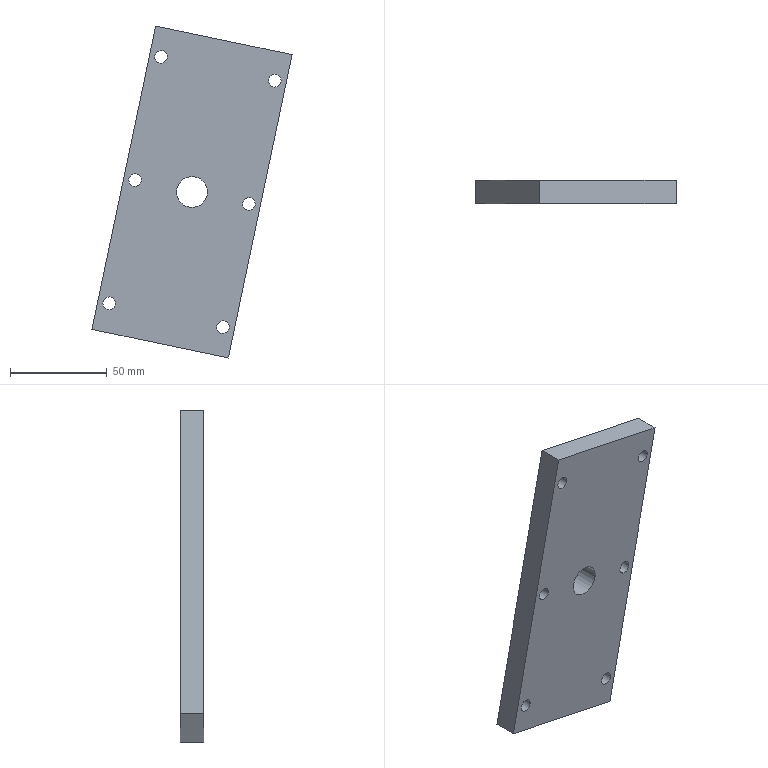Part | STEP file | SN10_007_001-03_PLACA | 1 solid | 13 faces | box 103.364 x 12 x 171.387 mm | volume 133438 mm3 | cylinder 7 | plane 6 | commonest cylinder face diameters 6.5 x6 16 x1
STEP:
#1=CARTESIAN_POINT('',(0.,0.,0.));
#2=DIRECTION('',(0.,0.,1.));
#3=DIRECTION('',(1.,0.,0.));
#4=AXIS2_PLACEMENT_3D('',#1,#2,#3);
#5=CARTESIAN_POINT('',(-608.399,-875.15,536.206));
#6=VERTEX_POINT('',#5);
#7=CARTESIAN_POINT('',(-592.741,-875.15,532.916));
#8=VERTEX_POINT('',#7);
#9=CARTESIAN_POINT('',(-600.57,-875.15,534.561));
#10=DIRECTION('',(0.,1.,0.));
#11=DIRECTION('',(0.9786,0.,-0.2056));
#12=AXIS2_PLACEMENT_3D('',#9,#10,#11);
#13=CIRCLE('',#12,8.);
#14=CARTESIAN_POINT('',(-600.57,-1063.653,534.561));
#15=DIRECTION('',(0.,1.,0.));
#16=DIRECTION('',(0.9786,0.,-0.2056));
#17=AXIS2_PLACEMENT_3D('',#14,#15,#16);
#18=CYLINDRICAL_SURFACE('',#17,8.);
#19=CARTESIAN_POINT('',(0.,188.503));
#20=DIRECTION('',(1.,0.));
#21=VECTOR('',#20,1.);
#22=LINE('',#19,#21);
#23=(GEOMETRIC_REPRESENTATION_CONTEXT(2)PARAMETRIC_REPRESENTATION_CONTEXT()REPRESENTATION_CONTEXT('',''));
#24=DEFINITIONAL_REPRESENTATION('',(#22),#23);
#25=PCURVE('',#18,#24);
#26=CARTESIAN_POINT('',(0.,-875.15,0.));
#27=DIRECTION('',(0.,1.,0.));
#28=DIRECTION('',(0.,0.,1.));
#29=AXIS2_PLACEMENT_3D('',#26,#27,#28);
#30=PLANE('',#29);
#31=CARTESIAN_POINT('',(534.561,-600.57));
#32=DIRECTION('',(-0.2056,0.9786));
#33=AXIS2_PLACEMENT_2D('',#31,#32);
#34=CIRCLE('',#33,8.);
#35=(GEOMETRIC_REPRESENTATION_CONTEXT(2)PARAMETRIC_REPRESENTATION_CONTEXT()REPRESENTATION_CONTEXT('',''));
#36=DEFINITIONAL_REPRESENTATION('',(#34),#35);
#37=PCURVE('',#30,#36);
#38=SURFACE_CURVE('',#13,(#25,#37),.PCURVE_S1.);
#39=EDGE_CURVE('',#6,#8,#38,.T.);
#40=ORIENTED_EDGE('',*,*,#39,.T.);
#41=CARTESIAN_POINT('',(-592.741,-863.15,532.916));
#42=VERTEX_POINT('',#41);
#43=CARTESIAN_POINT('',(-592.741,-875.15,532.916));
#44=CARTESIAN_POINT('',(-592.741,-863.15,532.916));
#45=B_SPLINE_CURVE_WITH_KNOTS('',1,(#43,#44),.UNSPECIFIED.,.F.,.F.,(2,2),(188.503,200.503),.PIECEWISE_BEZIER_KNOTS.);
#46=CARTESIAN_POINT('',(6.283,0.));
#47=DIRECTION('',(0.,1.));
#48=VECTOR('',#47,1.);
#49=LINE('',#46,#48);
#50=(GEOMETRIC_REPRESENTATION_CONTEXT(2)PARAMETRIC_REPRESENTATION_CONTEXT()REPRESENTATION_CONTEXT('',''));
#51=DEFINITIONAL_REPRESENTATION('',(#49),#50);
#52=PCURVE('',#18,#51);
#53=CARTESIAN_POINT('',(0.,0.));
#54=DIRECTION('',(0.,1.));
#55=VECTOR('',#54,1.);
#56=LINE('',#53,#55);
#57=(GEOMETRIC_REPRESENTATION_CONTEXT(2)PARAMETRIC_REPRESENTATION_CONTEXT()REPRESENTATION_CONTEXT('',''));
#58=DEFINITIONAL_REPRESENTATION('',(#56),#57);
#59=PCURVE('',#18,#58);
#60=SEAM_CURVE('',#45,(#52,#59),.PCURVE_S1.);
#61=EDGE_CURVE('',#8,#42,#60,.T.);
#62=ORIENTED_EDGE('',*,*,#61,.T.);
#63=CARTESIAN_POINT('',(-600.57,-863.15,534.561));
#64=DIRECTION('',(0.,-1.,0.));
#65=DIRECTION('',(0.9786,0.,-0.2056));
#66=AXIS2_PLACEMENT_3D('',#63,#64,#65);
#67=CIRCLE('',#66,8.);
#68=CARTESIAN_POINT('',(6.283,200.503));
#69=DIRECTION('',(-1.,0.));
#70=VECTOR('',#69,1.);
#71=LINE('',#68,#70);
#72=(GEOMETRIC_REPRESENTATION_CONTEXT(2)PARAMETRIC_REPRESENTATION_CONTEXT()REPRESENTATION_CONTEXT('',''));
#73=DEFINITIONAL_REPRESENTATION('',(#71),#72);
#74=PCURVE('',#18,#73);
#75=CARTESIAN_POINT('',(-541.059,-863.15,603.803));
#76=DIRECTION('',(0.,1.,0.));
#77=DIRECTION('',(0.,0.,1.));
#78=AXIS2_PLACEMENT_3D('',#75,#76,#77);
#79=PLANE('',#78);
#80=CARTESIAN_POINT('',(-70.887,-51.682));
#81=CARTESIAN_POINT('',(-57.327,-48.833));
#82=CARTESIAN_POINT('',(-61.639,-62.001));
#83=CARTESIAN_POINT('',(-65.952,-75.169));
#84=CARTESIAN_POINT('',(-75.199,-64.85));
#85=CARTESIAN_POINT('',(-84.447,-54.532));
#86=CARTESIAN_POINT('',(-70.887,-51.682));
#87=(BOUNDED_CURVE()B_SPLINE_CURVE(2,(#80,#81,#82,#83,#84,#85,#86),.UNSPECIFIED.,.T.,.F.)B_SPLINE_CURVE_WITH_KNOTS((1,2,2,2,2,1),(-2.094,0.,2.094,4.189,6.283,8.378),.UNSPECIFIED.)CURVE()GEOMETRIC_REPRESENTATION_ITEM()RATIONAL_B_SPLINE_CURVE((1.,0.5,1.,0.5,1.,0.5,1.))REPRESENTATION_ITEM(''));
#88=(GEOMETRIC_REPRESENTATION_CONTEXT(2)PARAMETRIC_REPRESENTATION_CONTEXT()REPRESENTATION_CONTEXT('',''));
#89=DEFINITIONAL_REPRESENTATION('',(#87),#88);
#90=PCURVE('',#79,#89);
#91=SURFACE_CURVE('',#67,(#74,#90),.PCURVE_S1.);
#92=EDGE_CURVE('',#42,#42,#91,.T.);
#93=ORIENTED_EDGE('',*,*,#92,.T.);
#94=ORIENTED_EDGE('',*,*,#61,.F.);
#95=CARTESIAN_POINT('',(-600.57,-875.15,534.561));
#96=DIRECTION('',(0.,1.,0.));
#97=DIRECTION('',(0.9786,0.,-0.2056));
#98=AXIS2_PLACEMENT_3D('',#95,#96,#97);
#99=CIRCLE('',#98,8.);
#100=CARTESIAN_POINT('',(-6.283,188.503));
#101=DIRECTION('',(1.,0.));
#102=VECTOR('',#101,1.);
#103=LINE('',#100,#102);
#104=(GEOMETRIC_REPRESENTATION_CONTEXT(2)PARAMETRIC_REPRESENTATION_CONTEXT()REPRESENTATION_CONTEXT('',''));
#105=DEFINITIONAL_REPRESENTATION('',(#103),#104);
#106=PCURVE('',#18,#105);
#107=CARTESIAN_POINT('',(534.561,-600.57));
#108=DIRECTION('',(-0.2056,0.9786));
#109=AXIS2_PLACEMENT_2D('',#107,#108);
#110=CIRCLE('',#109,8.);
#111=(GEOMETRIC_REPRESENTATION_CONTEXT(2)PARAMETRIC_REPRESENTATION_CONTEXT()REPRESENTATION_CONTEXT('',''));
#112=DEFINITIONAL_REPRESENTATION('',(#110),#111);
#113=PCURVE('',#30,#112);
#114=SURFACE_CURVE('',#99,(#106,#113),.PCURVE_S1.);
#115=EDGE_CURVE('',#8,#6,#114,.T.);
#116=ORIENTED_EDGE('',*,*,#115,.T.);
#117=EDGE_LOOP('',(#40,#62,#93,#94,#116));
#118=FACE_BOUND('',#117,.F.);
#119=ADVANCED_FACE('',(#118),#18,.F.);
#120=CARTESIAN_POINT('',(-587.759,-863.15,465.449));
#121=VERTEX_POINT('',#120);
#122=CARTESIAN_POINT('',(-581.398,-863.15,464.113));
#123=VERTEX_POINT('',#122);
#124=CARTESIAN_POINT('',(-584.578,-863.15,464.781));
#125=DIRECTION('',(0.,-1.,0.));
#126=DIRECTION('',(0.9786,0.,-0.2056));
#127=AXIS2_PLACEMENT_3D('',#124,#125,#126);
#128=CIRCLE('',#127,3.25);
#129=CARTESIAN_POINT('',(-584.578,-674.647,464.781));
#130=DIRECTION('',(0.,-1.,0.));
#131=DIRECTION('',(0.9786,0.,-0.2056));
#132=AXIS2_PLACEMENT_3D('',#129,#130,#131);
#133=CYLINDRICAL_SURFACE('',#132,3.25);
#134=CARTESIAN_POINT('',(0.,188.503));
#135=DIRECTION('',(1.,0.));
#136=VECTOR('',#135,1.);
#137=LINE('',#134,#136);
#138=(GEOMETRIC_REPRESENTATION_CONTEXT(2)PARAMETRIC_REPRESENTATION_CONTEXT()REPRESENTATION_CONTEXT('',''));
#139=DEFINITIONAL_REPRESENTATION('',(#137),#138);
#140=PCURVE('',#133,#139);
#141=CARTESIAN_POINT('',(-139.69,-40.339));
#142=CARTESIAN_POINT('',(-134.181,-39.181));
#143=CARTESIAN_POINT('',(-135.933,-44.531));
#144=CARTESIAN_POINT('',(-137.685,-49.88));
#145=CARTESIAN_POINT('',(-141.442,-45.688));
#146=CARTESIAN_POINT('',(-145.199,-41.496));
#147=CARTESIAN_POINT('',(-139.69,-40.339));
#148=(BOUNDED_CURVE()B_SPLINE_CURVE(2,(#141,#142,#143,#144,#145,#146,#147),.UNSPECIFIED.,.T.,.F.)B_SPLINE_CURVE_WITH_KNOTS((1,2,2,2,2,1),(-2.094,0.,2.094,4.189,6.283,8.378),.UNSPECIFIED.)CURVE()GEOMETRIC_REPRESENTATION_ITEM()RATIONAL_B_SPLINE_CURVE((1.,0.5,1.,0.5,1.,0.5,1.))REPRESENTATION_ITEM(''));
#149=(GEOMETRIC_REPRESENTATION_CONTEXT(2)PARAMETRIC_REPRESENTATION_CONTEXT()REPRESENTATION_CONTEXT('',''));
#150=DEFINITIONAL_REPRESENTATION('',(#148),#149);
#151=PCURVE('',#79,#150);
#152=SURFACE_CURVE('',#128,(#140,#151),.PCURVE_S1.);
#153=EDGE_CURVE('',#121,#123,#152,.T.);
#154=ORIENTED_EDGE('',*,*,#153,.T.);
#155=CARTESIAN_POINT('',(-581.398,-875.15,464.113));
#156=VERTEX_POINT('',#155);
#157=CARTESIAN_POINT('',(-581.398,-863.15,464.113));
#158=CARTESIAN_POINT('',(-581.398,-875.15,464.113));
#159=B_SPLINE_CURVE_WITH_KNOTS('',1,(#157,#158),.UNSPECIFIED.,.F.,.F.,(2,2),(188.503,200.503),.PIECEWISE_BEZIER_KNOTS.);
#160=CARTESIAN_POINT('',(6.283,0.));
#161=DIRECTION('',(0.,1.));
#162=VECTOR('',#161,1.);
#163=LINE('',#160,#162);
#164=(GEOMETRIC_REPRESENTATION_CONTEXT(2)PARAMETRIC_REPRESENTATION_CONTEXT()REPRESENTATION_CONTEXT('',''));
#165=DEFINITIONAL_REPRESENTATION('',(#163),#164);
#166=PCURVE('',#133,#165);
#167=CARTESIAN_POINT('',(0.,0.));
#168=DIRECTION('',(0.,1.));
#169=VECTOR('',#168,1.);
#170=LINE('',#167,#169);
#171=(GEOMETRIC_REPRESENTATION_CONTEXT(2)PARAMETRIC_REPRESENTATION_CONTEXT()REPRESENTATION_CONTEXT('',''));
#172=DEFINITIONAL_REPRESENTATION('',(#170),#171);
#173=PCURVE('',#133,#172);
#174=SEAM_CURVE('',#159,(#166,#173),.PCURVE_S1.);
#175=EDGE_CURVE('',#123,#156,#174,.T.);
#176=ORIENTED_EDGE('',*,*,#175,.T.);
#177=CARTESIAN_POINT('',(-584.578,-875.15,464.781));
#178=DIRECTION('',(0.,1.,0.));
#179=DIRECTION('',(0.9786,0.,-0.2056));
#180=AXIS2_PLACEMENT_3D('',#177,#178,#179);
#181=CIRCLE('',#180,3.25);
#182=CARTESIAN_POINT('',(6.283,200.503));
#183=DIRECTION('',(-1.,0.));
#184=VECTOR('',#183,1.);
#185=LINE('',#182,#184);
#186=(GEOMETRIC_REPRESENTATION_CONTEXT(2)PARAMETRIC_REPRESENTATION_CONTEXT()REPRESENTATION_CONTEXT('',''));
#187=DEFINITIONAL_REPRESENTATION('',(#185),#186);
#188=PCURVE('',#133,#187);
#189=CARTESIAN_POINT('',(464.781,-584.578));
#190=DIRECTION('',(-0.2056,0.9786));
#191=AXIS2_PLACEMENT_2D('',#189,#190);
#192=CIRCLE('',#191,3.25);
#193=(GEOMETRIC_REPRESENTATION_CONTEXT(2)PARAMETRIC_REPRESENTATION_CONTEXT()REPRESENTATION_CONTEXT('',''));
#194=DEFINITIONAL_REPRESENTATION('',(#192),#193);
#195=PCURVE('',#30,#194);
#196=SURFACE_CURVE('',#181,(#188,#195),.PCURVE_S1.);
#197=EDGE_CURVE('',#156,#156,#196,.T.);
#198=ORIENTED_EDGE('',*,*,#197,.T.);
#199=ORIENTED_EDGE('',*,*,#175,.F.);
#200=CARTESIAN_POINT('',(-584.578,-863.15,464.781));
#201=DIRECTION('',(0.,-1.,0.));
#202=DIRECTION('',(0.9786,0.,-0.2056));
#203=AXIS2_PLACEMENT_3D('',#200,#201,#202);
#204=CIRCLE('',#203,3.25);
#205=CARTESIAN_POINT('',(-6.283,188.503));
#206=DIRECTION('',(1.,0.));
#207=VECTOR('',#206,1.);
#208=LINE('',#205,#207);
#209=(GEOMETRIC_REPRESENTATION_CONTEXT(2)PARAMETRIC_REPRESENTATION_CONTEXT()REPRESENTATION_CONTEXT('',''));
#210=DEFINITIONAL_REPRESENTATION('',(#208),#209);
#211=PCURVE('',#133,#210);
#212=CARTESIAN_POINT('',(-139.69,-40.339));
#213=CARTESIAN_POINT('',(-134.181,-39.181));
#214=CARTESIAN_POINT('',(-135.933,-44.531));
#215=CARTESIAN_POINT('',(-137.685,-49.88));
#216=CARTESIAN_POINT('',(-141.442,-45.688));
#217=CARTESIAN_POINT('',(-145.199,-41.496));
#218=CARTESIAN_POINT('',(-139.69,-40.339));
#219=(BOUNDED_CURVE()B_SPLINE_CURVE(2,(#212,#213,#214,#215,#216,#217,#218),.UNSPECIFIED.,.T.,.F.)B_SPLINE_CURVE_WITH_KNOTS((1,2,2,2,2,1),(-2.094,0.,2.094,4.189,6.283,8.378),.UNSPECIFIED.)CURVE()GEOMETRIC_REPRESENTATION_ITEM()RATIONAL_B_SPLINE_CURVE((1.,0.5,1.,0.5,1.,0.5,1.))REPRESENTATION_ITEM(''));
#220=(GEOMETRIC_REPRESENTATION_CONTEXT(2)PARAMETRIC_REPRESENTATION_CONTEXT()REPRESENTATION_CONTEXT('',''));
#221=DEFINITIONAL_REPRESENTATION('',(#219),#220);
#222=PCURVE('',#79,#221);
#223=SURFACE_CURVE('',#204,(#211,#222),.PCURVE_S1.);
#224=EDGE_CURVE('',#123,#121,#223,.T.);
#225=ORIENTED_EDGE('',*,*,#224,.T.);
#226=EDGE_LOOP('',(#154,#176,#198,#199,#225));
#227=FACE_BOUND('',#226,.F.);
#228=ADVANCED_FACE('',(#227),#133,.F.);
#229=CARTESIAN_POINT('',(-574.392,-863.15,529.06));
#230=VERTEX_POINT('',#229);
#231=CARTESIAN_POINT('',(-568.031,-863.15,527.723));
#232=VERTEX_POINT('',#231);
#233=CARTESIAN_POINT('',(-571.211,-863.15,528.392));
#234=DIRECTION('',(0.,-1.,0.));
#235=DIRECTION('',(0.9786,0.,-0.2056));
#236=AXIS2_PLACEMENT_3D('',#233,#234,#235);
#237=CIRCLE('',#236,3.25);
#238=CARTESIAN_POINT('',(-571.211,-674.647,528.392));
#239=DIRECTION('',(0.,-1.,0.));
#240=DIRECTION('',(0.9786,0.,-0.2056));
#241=AXIS2_PLACEMENT_3D('',#238,#239,#240);
#242=CYLINDRICAL_SURFACE('',#241,3.25);
#243=CARTESIAN_POINT('',(0.,188.503));
#244=DIRECTION('',(1.,0.));
#245=VECTOR('',#244,1.);
#246=LINE('',#243,#245);
#247=(GEOMETRIC_REPRESENTATION_CONTEXT(2)PARAMETRIC_REPRESENTATION_CONTEXT()REPRESENTATION_CONTEXT('',''));
#248=DEFINITIONAL_REPRESENTATION('',(#246),#247);
#249=PCURVE('',#242,#248);
#250=CARTESIAN_POINT('',(-76.079,-26.972));
#251=CARTESIAN_POINT('',(-70.571,-25.814));
#252=CARTESIAN_POINT('',(-72.323,-31.164));
#253=CARTESIAN_POINT('',(-74.074,-36.513));
#254=CARTESIAN_POINT('',(-77.831,-32.321));
#255=CARTESIAN_POINT('',(-81.588,-28.129));
#256=CARTESIAN_POINT('',(-76.079,-26.972));
#257=(BOUNDED_CURVE()B_SPLINE_CURVE(2,(#250,#251,#252,#253,#254,#255,#256),.UNSPECIFIED.,.T.,.F.)B_SPLINE_CURVE_WITH_KNOTS((1,2,2,2,2,1),(-2.094,0.,2.094,4.189,6.283,8.378),.UNSPECIFIED.)CURVE()GEOMETRIC_REPRESENTATION_ITEM()RATIONAL_B_SPLINE_CURVE((1.,0.5,1.,0.5,1.,0.5,1.))REPRESENTATION_ITEM(''));
#258=(GEOMETRIC_REPRESENTATION_CONTEXT(2)PARAMETRIC_REPRESENTATION_CONTEXT()REPRESENTATION_CONTEXT('',''));
#259=DEFINITIONAL_REPRESENTATION('',(#257),#258);
#260=PCURVE('',#79,#259);
#261=SURFACE_CURVE('',#237,(#249,#260),.PCURVE_S1.);
#262=EDGE_CURVE('',#230,#232,#261,.T.);
#263=ORIENTED_EDGE('',*,*,#262,.T.);
#264=CARTESIAN_POINT('',(-568.031,-875.15,527.723));
#265=VERTEX_POINT('',#264);
#266=CARTESIAN_POINT('',(-568.031,-863.15,527.723));
#267=CARTESIAN_POINT('',(-568.031,-875.15,527.723));
#268=B_SPLINE_CURVE_WITH_KNOTS('',1,(#266,#267),.UNSPECIFIED.,.F.,.F.,(2,2),(188.503,200.503),.PIECEWISE_BEZIER_KNOTS.);
#269=CARTESIAN_POINT('',(6.283,0.));
#270=DIRECTION('',(0.,1.));
#271=VECTOR('',#270,1.);
#272=LINE('',#269,#271);
#273=(GEOMETRIC_REPRESENTATION_CONTEXT(2)PARAMETRIC_REPRESENTATION_CONTEXT()REPRESENTATION_CONTEXT('',''));
#274=DEFINITIONAL_REPRESENTATION('',(#272),#273);
#275=PCURVE('',#242,#274);
#276=CARTESIAN_POINT('',(0.,0.));
#277=DIRECTION('',(0.,1.));
#278=VECTOR('',#277,1.);
#279=LINE('',#276,#278);
#280=(GEOMETRIC_REPRESENTATION_CONTEXT(2)PARAMETRIC_REPRESENTATION_CONTEXT()REPRESENTATION_CONTEXT('',''));
#281=DEFINITIONAL_REPRESENTATION('',(#279),#280);
#282=PCURVE('',#242,#281);
#283=SEAM_CURVE('',#268,(#275,#282),.PCURVE_S1.);
#284=EDGE_CURVE('',#232,#265,#283,.T.);
#285=ORIENTED_EDGE('',*,*,#284,.T.);
#286=CARTESIAN_POINT('',(-571.211,-875.15,528.392));
#287=DIRECTION('',(0.,1.,0.));
#288=DIRECTION('',(0.9786,0.,-0.2056));
#289=AXIS2_PLACEMENT_3D('',#286,#287,#288);
#290=CIRCLE('',#289,3.25);
#291=CARTESIAN_POINT('',(6.283,200.503));
#292=DIRECTION('',(-1.,0.));
#293=VECTOR('',#292,1.);
#294=LINE('',#291,#293);
#295=(GEOMETRIC_REPRESENTATION_CONTEXT(2)PARAMETRIC_REPRESENTATION_CONTEXT()REPRESENTATION_CONTEXT('',''));
#296=DEFINITIONAL_REPRESENTATION('',(#294),#295);
#297=PCURVE('',#242,#296);
#298=CARTESIAN_POINT('',(528.392,-571.211));
#299=DIRECTION('',(-0.2056,0.9786));
#300=AXIS2_PLACEMENT_2D('',#298,#299);
#301=CIRCLE('',#300,3.25);
#302=(GEOMETRIC_REPRESENTATION_CONTEXT(2)PARAMETRIC_REPRESENTATION_CONTEXT()REPRESENTATION_CONTEXT('',''));
#303=DEFINITIONAL_REPRESENTATION('',(#301),#302);
#304=PCURVE('',#30,#303);
#305=SURFACE_CURVE('',#290,(#297,#304),.PCURVE_S1.);
#306=EDGE_CURVE('',#265,#265,#305,.T.);
#307=ORIENTED_EDGE('',*,*,#306,.T.);
#308=ORIENTED_EDGE('',*,*,#284,.F.);
#309=CARTESIAN_POINT('',(-571.211,-863.15,528.392));
#310=DIRECTION('',(0.,-1.,0.));
#311=DIRECTION('',(0.9786,0.,-0.2056));
#312=AXIS2_PLACEMENT_3D('',#309,#310,#311);
#313=CIRCLE('',#312,3.25);
#314=CARTESIAN_POINT('',(-6.283,188.503));
#315=DIRECTION('',(1.,0.));
#316=VECTOR('',#315,1.);
#317=LINE('',#314,#316);
#318=(GEOMETRIC_REPRESENTATION_CONTEXT(2)PARAMETRIC_REPRESENTATION_CONTEXT()REPRESENTATION_CONTEXT('',''));
#319=DEFINITIONAL_REPRESENTATION('',(#317),#318);
#320=PCURVE('',#242,#319);
#321=CARTESIAN_POINT('',(-76.079,-26.972));
#322=CARTESIAN_POINT('',(-70.571,-25.814));
#323=CARTESIAN_POINT('',(-72.323,-31.164));
#324=CARTESIAN_POINT('',(-74.074,-36.513));
#325=CARTESIAN_POINT('',(-77.831,-32.321));
#326=CARTESIAN_POINT('',(-81.588,-28.129));
#327=CARTESIAN_POINT('',(-76.079,-26.972));
#328=(BOUNDED_CURVE()B_SPLINE_CURVE(2,(#321,#322,#323,#324,#325,#326,#327),.UNSPECIFIED.,.T.,.F.)B_SPLINE_CURVE_WITH_KNOTS((1,2,2,2,2,1),(-2.094,0.,2.094,4.189,6.283,8.378),.UNSPECIFIED.)CURVE()GEOMETRIC_REPRESENTATION_ITEM()RATIONAL_B_SPLINE_CURVE((1.,0.5,1.,0.5,1.,0.5,1.))REPRESENTATION_ITEM(''));
#329=(GEOMETRIC_REPRESENTATION_CONTEXT(2)PARAMETRIC_REPRESENTATION_CONTEXT()REPRESENTATION_CONTEXT('',''));
#330=DEFINITIONAL_REPRESENTATION('',(#328),#329);
#331=PCURVE('',#79,#330);
#332=SURFACE_CURVE('',#313,(#320,#331),.PCURVE_S1.);
#333=EDGE_CURVE('',#232,#230,#332,.T.);
#334=ORIENTED_EDGE('',*,*,#333,.T.);
#335=EDGE_LOOP('',(#263,#285,#307,#308,#334));
#336=FACE_BOUND('',#335,.F.);
#337=ADVANCED_FACE('',(#336),#242,.F.);
#338=CARTESIAN_POINT('',(-561.025,-863.15,592.671));
#339=VERTEX_POINT('',#338);
#340=CARTESIAN_POINT('',(-554.664,-863.15,591.334));
#341=VERTEX_POINT('',#340);
#342=CARTESIAN_POINT('',(-557.845,-863.15,592.003));
#343=DIRECTION('',(0.,-1.,0.));
#344=DIRECTION('',(0.9786,0.,-0.2056));
#345=AXIS2_PLACEMENT_3D('',#342,#343,#344);
#346=CIRCLE('',#345,3.25);
#347=CARTESIAN_POINT('',(-557.845,-674.647,592.003));
#348=DIRECTION('',(0.,-1.,0.));
#349=DIRECTION('',(0.9786,0.,-0.2056));
#350=AXIS2_PLACEMENT_3D('',#347,#348,#349);
#351=CYLINDRICAL_SURFACE('',#350,3.25);
#352=CARTESIAN_POINT('',(0.,188.503));
#353=DIRECTION('',(1.,0.));
#354=VECTOR('',#353,1.);
#355=LINE('',#352,#354);
#356=(GEOMETRIC_REPRESENTATION_CONTEXT(2)PARAMETRIC_REPRESENTATION_CONTEXT()REPRESENTATION_CONTEXT('',''));
#357=DEFINITIONAL_REPRESENTATION('',(#355),#356);
#358=PCURVE('',#351,#357);
#359=CARTESIAN_POINT('',(-12.469,-13.605));
#360=CARTESIAN_POINT('',(-6.96,-12.447));
#361=CARTESIAN_POINT('',(-8.712,-17.797));
#362=CARTESIAN_POINT('',(-10.464,-23.147));
#363=CARTESIAN_POINT('',(-14.221,-18.954));
#364=CARTESIAN_POINT('',(-17.978,-14.762));
#365=CARTESIAN_POINT('',(-12.469,-13.605));
#366=(BOUNDED_CURVE()B_SPLINE_CURVE(2,(#359,#360,#361,#362,#363,#364,#365),.UNSPECIFIED.,.T.,.F.)B_SPLINE_CURVE_WITH_KNOTS((1,2,2,2,2,1),(-2.094,0.,2.094,4.189,6.283,8.378),.UNSPECIFIED.)CURVE()GEOMETRIC_REPRESENTATION_ITEM()RATIONAL_B_SPLINE_CURVE((1.,0.5,1.,0.5,1.,0.5,1.))REPRESENTATION_ITEM(''));
#367=(GEOMETRIC_REPRESENTATION_CONTEXT(2)PARAMETRIC_REPRESENTATION_CONTEXT()REPRESENTATION_CONTEXT('',''));
#368=DEFINITIONAL_REPRESENTATION('',(#366),#367);
#369=PCURVE('',#79,#368);
#370=SURFACE_CURVE('',#346,(#358,#369),.PCURVE_S1.);
#371=EDGE_CURVE('',#339,#341,#370,.T.);
#372=ORIENTED_EDGE('',*,*,#371,.T.);
#373=CARTESIAN_POINT('',(-554.664,-875.15,591.334));
#374=VERTEX_POINT('',#373);
#375=CARTESIAN_POINT('',(-554.664,-863.15,591.334));
#376=CARTESIAN_POINT('',(-554.664,-875.15,591.334));
#377=B_SPLINE_CURVE_WITH_KNOTS('',1,(#375,#376),.UNSPECIFIED.,.F.,.F.,(2,2),(188.503,200.503),.PIECEWISE_BEZIER_KNOTS.);
#378=CARTESIAN_POINT('',(6.283,0.));
#379=DIRECTION('',(0.,1.));
#380=VECTOR('',#379,1.);
#381=LINE('',#378,#380);
#382=(GEOMETRIC_REPRESENTATION_CONTEXT(2)PARAMETRIC_REPRESENTATION_CONTEXT()REPRESENTATION_CONTEXT('',''));
#383=DEFINITIONAL_REPRESENTATION('',(#381),#382);
#384=PCURVE('',#351,#383);
#385=CARTESIAN_POINT('',(0.,0.));
#386=DIRECTION('',(0.,1.));
#387=VECTOR('',#386,1.);
#388=LINE('',#385,#387);
#389=(GEOMETRIC_REPRESENTATION_CONTEXT(2)PARAMETRIC_REPRESENTATION_CONTEXT()REPRESENTATION_CONTEXT('',''));
#390=DEFINITIONAL_REPRESENTATION('',(#388),#389);
#391=PCURVE('',#351,#390);
#392=SEAM_CURVE('',#377,(#384,#391),.PCURVE_S1.);
#393=EDGE_CURVE('',#341,#374,#392,.T.);
#394=ORIENTED_EDGE('',*,*,#393,.T.);
#395=CARTESIAN_POINT('',(-557.845,-875.15,592.003));
#396=DIRECTION('',(0.,1.,0.));
#397=DIRECTION('',(0.9786,0.,-0.2056));
#398=AXIS2_PLACEMENT_3D('',#395,#396,#397);
#399=CIRCLE('',#398,3.25);
#400=CARTESIAN_POINT('',(6.283,200.503));
#401=DIRECTION('',(-1.,0.));
#402=VECTOR('',#401,1.);
#403=LINE('',#400,#402);
#404=(GEOMETRIC_REPRESENTATION_CONTEXT(2)PARAMETRIC_REPRESENTATION_CONTEXT()REPRESENTATION_CONTEXT('',''));
#405=DEFINITIONAL_REPRESENTATION('',(#403),#404);
#406=PCURVE('',#351,#405);
#407=CARTESIAN_POINT('',(592.003,-557.845));
#408=DIRECTION('',(-0.2056,0.9786));
#409=AXIS2_PLACEMENT_2D('',#407,#408);
#410=CIRCLE('',#409,3.25);
#411=(GEOMETRIC_REPRESENTATION_CONTEXT(2)PARAMETRIC_REPRESENTATION_CONTEXT()REPRESENTATION_CONTEXT('',''));
#412=DEFINITIONAL_REPRESENTATION('',(#410),#411);
#413=PCURVE('',#30,#412);
#414=SURFACE_CURVE('',#399,(#406,#413),.PCURVE_S1.);
#415=EDGE_CURVE('',#374,#374,#414,.T.);
#416=ORIENTED_EDGE('',*,*,#415,.T.);
#417=ORIENTED_EDGE('',*,*,#393,.F.);
#418=CARTESIAN_POINT('',(-557.845,-863.15,592.003));
#419=DIRECTION('',(0.,-1.,0.));
#420=DIRECTION('',(0.9786,0.,-0.2056));
#421=AXIS2_PLACEMENT_3D('',#418,#419,#420);
#422=CIRCLE('',#421,3.25);
#423=CARTESIAN_POINT('',(-6.283,188.503));
#424=DIRECTION('',(1.,0.));
#425=VECTOR('',#424,1.);
#426=LINE('',#423,#425);
#427=(GEOMETRIC_REPRESENTATION_CONTEXT(2)PARAMETRIC_REPRESENTATION_CONTEXT()REPRESENTATION_CONTEXT('',''));
#428=DEFINITIONAL_REPRESENTATION('',(#426),#427);
#429=PCURVE('',#351,#428);
#430=CARTESIAN_POINT('',(-12.469,-13.605));
#431=CARTESIAN_POINT('',(-6.96,-12.447));
#432=CARTESIAN_POINT('',(-8.712,-17.797));
#433=CARTESIAN_POINT('',(-10.464,-23.147));
#434=CARTESIAN_POINT('',(-14.221,-18.954));
#435=CARTESIAN_POINT('',(-17.978,-14.762));
#436=CARTESIAN_POINT('',(-12.469,-13.605));
#437=(BOUNDED_CURVE()B_SPLINE_CURVE(2,(#430,#431,#432,#433,#434,#435,#436),.UNSPECIFIED.,.T.,.F.)B_SPLINE_CURVE_WITH_KNOTS((1,2,2,2,2,1),(-2.094,0.,2.094,4.189,6.283,8.378),.UNSPECIFIED.)CURVE()GEOMETRIC_REPRESENTATION_ITEM()RATIONAL_B_SPLINE_CURVE((1.,0.5,1.,0.5,1.,0.5,1.))REPRESENTATION_ITEM(''));
#438=(GEOMETRIC_REPRESENTATION_CONTEXT(2)PARAMETRIC_REPRESENTATION_CONTEXT()REPRESENTATION_CONTEXT('',''));
#439=DEFINITIONAL_REPRESENTATION('',(#437),#438);
#440=PCURVE('',#79,#439);
#441=SURFACE_CURVE('',#422,(#429,#440),.PCURVE_S1.);
#442=EDGE_CURVE('',#341,#339,#441,.T.);
#443=ORIENTED_EDGE('',*,*,#442,.T.);
#444=EDGE_LOOP('',(#372,#394,#416,#417,#443));
#445=FACE_BOUND('',#444,.F.);
#446=ADVANCED_FACE('',(#445),#351,.F.);
#447=CARTESIAN_POINT('',(-633.11,-863.15,541.399));
#448=VERTEX_POINT('',#447);
#449=CARTESIAN_POINT('',(-626.748,-863.15,540.062));
#450=VERTEX_POINT('',#449);
#451=CARTESIAN_POINT('',(-629.929,-863.15,540.73));
#452=DIRECTION('',(0.,-1.,0.));
#453=DIRECTION('',(0.9786,0.,-0.2056));
#454=AXIS2_PLACEMENT_3D('',#451,#452,#453);
#455=CIRCLE('',#454,3.25);
#456=CARTESIAN_POINT('',(-629.929,-674.647,540.73));
#457=DIRECTION('',(0.,-1.,0.));
#458=DIRECTION('',(0.9786,0.,-0.2056));
#459=AXIS2_PLACEMENT_3D('',#456,#457,#458);
#460=CYLINDRICAL_SURFACE('',#459,3.25);
#461=CARTESIAN_POINT('',(0.,188.503));
#462=DIRECTION('',(1.,0.));
#463=VECTOR('',#462,1.);
#464=LINE('',#461,#463);
#465=(GEOMETRIC_REPRESENTATION_CONTEXT(2)PARAMETRIC_REPRESENTATION_CONTEXT()REPRESENTATION_CONTEXT('',''));
#466=DEFINITIONAL_REPRESENTATION('',(#464),#465);
#467=PCURVE('',#460,#466);
#468=CARTESIAN_POINT('',(-63.741,-85.689));
#469=CARTESIAN_POINT('',(-58.232,-84.532));
#470=CARTESIAN_POINT('',(-59.984,-89.881));
#471=CARTESIAN_POINT('',(-61.736,-95.231));
#472=CARTESIAN_POINT('',(-65.493,-91.039));
#473=CARTESIAN_POINT('',(-69.25,-86.847));
#474=CARTESIAN_POINT('',(-63.741,-85.689));
#475=(BOUNDED_CURVE()B_SPLINE_CURVE(2,(#468,#469,#470,#471,#472,#473,#474),.UNSPECIFIED.,.T.,.F.)B_SPLINE_CURVE_WITH_KNOTS((1,2,2,2,2,1),(-2.094,0.,2.094,4.189,6.283,8.378),.UNSPECIFIED.)CURVE()GEOMETRIC_REPRESENTATION_ITEM()RATIONAL_B_SPLINE_CURVE((1.,0.5,1.,0.5,1.,0.5,1.))REPRESENTATION_ITEM(''));
#476=(GEOMETRIC_REPRESENTATION_CONTEXT(2)PARAMETRIC_REPRESENTATION_CONTEXT()REPRESENTATION_CONTEXT('',''));
#477=DEFINITIONAL_REPRESENTATION('',(#475),#476);
#478=PCURVE('',#79,#477);
#479=SURFACE_CURVE('',#455,(#467,#478),.PCURVE_S1.);
#480=EDGE_CURVE('',#448,#450,#479,.T.);
#481=ORIENTED_EDGE('',*,*,#480,.T.);
#482=CARTESIAN_POINT('',(-626.748,-875.15,540.062));
#483=VERTEX_POINT('',#482);
#484=CARTESIAN_POINT('',(-626.748,-863.15,540.062));
#485=CARTESIAN_POINT('',(-626.748,-875.15,540.062));
#486=B_SPLINE_CURVE_WITH_KNOTS('',1,(#484,#485),.UNSPECIFIED.,.F.,.F.,(2,2),(188.503,200.503),.PIECEWISE_BEZIER_KNOTS.);
#487=CARTESIAN_POINT('',(6.283,0.));
#488=DIRECTION('',(0.,1.));
#489=VECTOR('',#488,1.);
#490=LINE('',#487,#489);
#491=(GEOMETRIC_REPRESENTATION_CONTEXT(2)PARAMETRIC_REPRESENTATION_CONTEXT()REPRESENTATION_CONTEXT('',''));
#492=DEFINITIONAL_REPRESENTATION('',(#490),#491);
#493=PCURVE('',#460,#492);
#494=CARTESIAN_POINT('',(0.,0.));
#495=DIRECTION('',(0.,1.));
#496=VECTOR('',#495,1.);
#497=LINE('',#494,#496);
#498=(GEOMETRIC_REPRESENTATION_CONTEXT(2)PARAMETRIC_REPRESENTATION_CONTEXT()REPRESENTATION_CONTEXT('',''));
#499=DEFINITIONAL_REPRESENTATION('',(#497),#498);
#500=PCURVE('',#460,#499);
#501=SEAM_CURVE('',#486,(#493,#500),.PCURVE_S1.);
#502=EDGE_CURVE('',#450,#483,#501,.T.);
#503=ORIENTED_EDGE('',*,*,#502,.T.);
#504=CARTESIAN_POINT('',(-629.929,-875.15,540.73));
#505=DIRECTION('',(0.,1.,0.));
#506=DIRECTION('',(0.9786,0.,-0.2056));
#507=AXIS2_PLACEMENT_3D('',#504,#505,#506);
#508=CIRCLE('',#507,3.25);
#509=CARTESIAN_POINT('',(6.283,200.503));
#510=DIRECTION('',(-1.,0.));
#511=VECTOR('',#510,1.);
#512=LINE('',#509,#511);
#513=(GEOMETRIC_REPRESENTATION_CONTEXT(2)PARAMETRIC_REPRESENTATION_CONTEXT()REPRESENTATION_CONTEXT('',''));
#514=DEFINITIONAL_REPRESENTATION('',(#512),#513);
#515=PCURVE('',#460,#514);
#516=CARTESIAN_POINT('',(540.73,-629.929));
#517=DIRECTION('',(-0.2056,0.9786));
#518=AXIS2_PLACEMENT_2D('',#516,#517);
#519=CIRCLE('',#518,3.25);
#520=(GEOMETRIC_REPRESENTATION_CONTEXT(2)PARAMETRIC_REPRESENTATION_CONTEXT()REPRESENTATION_CONTEXT('',''));
#521=DEFINITIONAL_REPRESENTATION('',(#519),#520);
#522=PCURVE('',#30,#521);
#523=SURFACE_CURVE('',#508,(#515,#522),.PCURVE_S1.);
#524=EDGE_CURVE('',#483,#483,#523,.T.);
#525=ORIENTED_EDGE('',*,*,#524,.T.);
#526=ORIENTED_EDGE('',*,*,#502,.F.);
#527=CARTESIAN_POINT('',(-629.929,-863.15,540.73));
#528=DIRECTION('',(0.,-1.,0.));
#529=DIRECTION('',(0.9786,0.,-0.2056));
#530=AXIS2_PLACEMENT_3D('',#527,#528,#529);
#531=CIRCLE('',#530,3.25);
#532=CARTESIAN_POINT('',(-6.283,188.503));
#533=DIRECTION('',(1.,0.));
#534=VECTOR('',#533,1.);
#535=LINE('',#532,#534);
#536=(GEOMETRIC_REPRESENTATION_CONTEXT(2)PARAMETRIC_REPRESENTATION_CONTEXT()REPRESENTATION_CONTEXT('',''));
#537=DEFINITIONAL_REPRESENTATION('',(#535),#536);
#538=PCURVE('',#460,#537);
#539=CARTESIAN_POINT('',(-63.741,-85.689));
#540=CARTESIAN_POINT('',(-58.232,-84.532));
#541=CARTESIAN_POINT('',(-59.984,-89.881));
#542=CARTESIAN_POINT('',(-61.736,-95.231));
#543=CARTESIAN_POINT('',(-65.493,-91.039));
#544=CARTESIAN_POINT('',(-69.25,-86.847));
#545=CARTESIAN_POINT('',(-63.741,-85.689));
#546=(BOUNDED_CURVE()B_SPLINE_CURVE(2,(#539,#540,#541,#542,#543,#544,#545),.UNSPECIFIED.,.T.,.F.)B_SPLINE_CURVE_WITH_KNOTS((1,2,2,2,2,1),(-2.094,0.,2.094,4.189,6.283,8.378),.UNSPECIFIED.)CURVE()GEOMETRIC_REPRESENTATION_ITEM()RATIONAL_B_SPLINE_CURVE((1.,0.5,1.,0.5,1.,0.5,1.))REPRESENTATION_ITEM(''));
#547=(GEOMETRIC_REPRESENTATION_CONTEXT(2)PARAMETRIC_REPRESENTATION_CONTEXT()REPRESENTATION_CONTEXT('',''));
#548=DEFINITIONAL_REPRESENTATION('',(#546),#547);
#549=PCURVE('',#79,#548);
#550=SURFACE_CURVE('',#531,(#538,#549),.PCURVE_S1.);
#551=EDGE_CURVE('',#450,#448,#550,.T.);
#552=ORIENTED_EDGE('',*,*,#551,.T.);
#553=EDGE_LOOP('',(#481,#503,#525,#526,#552));
#554=FACE_BOUND('',#553,.F.);
#555=ADVANCED_FACE('',(#554),#460,.F.);
#556=CARTESIAN_POINT('',(-646.476,-863.15,477.788));
#557=VERTEX_POINT('',#556);
#558=CARTESIAN_POINT('',(-640.115,-863.15,476.451));
#559=VERTEX_POINT('',#558);
#560=CARTESIAN_POINT('',(-643.296,-863.15,477.12));
#561=DIRECTION('',(0.,-1.,0.));
#562=DIRECTION('',(0.9786,0.,-0.2056));
#563=AXIS2_PLACEMENT_3D('',#560,#561,#562);
#564=CIRCLE('',#563,3.25);
#565=CARTESIAN_POINT('',(-643.296,-674.647,477.12));
#566=DIRECTION('',(0.,-1.,0.));
#567=DIRECTION('',(0.9786,0.,-0.2056));
#568=AXIS2_PLACEMENT_3D('',#565,#566,#567);
#569=CYLINDRICAL_SURFACE('',#568,3.25);
#570=CARTESIAN_POINT('',(0.,188.503));
#571=DIRECTION('',(1.,0.));
#572=VECTOR('',#571,1.);
#573=LINE('',#570,#572);
#574=(GEOMETRIC_REPRESENTATION_CONTEXT(2)PARAMETRIC_REPRESENTATION_CONTEXT()REPRESENTATION_CONTEXT('',''));
#575=DEFINITIONAL_REPRESENTATION('',(#573),#574);
#576=PCURVE('',#569,#575);
#577=CARTESIAN_POINT('',(-127.352,-99.056));
#578=CARTESIAN_POINT('',(-121.843,-97.899));
#579=CARTESIAN_POINT('',(-123.595,-103.248));
#580=CARTESIAN_POINT('',(-125.347,-108.598));
#581=CARTESIAN_POINT('',(-129.104,-104.406));
#582=CARTESIAN_POINT('',(-132.861,-100.214));
#583=CARTESIAN_POINT('',(-127.352,-99.056));
#584=(BOUNDED_CURVE()B_SPLINE_CURVE(2,(#577,#578,#579,#580,#581,#582,#583),.UNSPECIFIED.,.T.,.F.)B_SPLINE_CURVE_WITH_KNOTS((1,2,2,2,2,1),(-2.094,0.,2.094,4.189,6.283,8.378),.UNSPECIFIED.)CURVE()GEOMETRIC_REPRESENTATION_ITEM()RATIONAL_B_SPLINE_CURVE((1.,0.5,1.,0.5,1.,0.5,1.))REPRESENTATION_ITEM(''));
#585=(GEOMETRIC_REPRESENTATION_CONTEXT(2)PARAMETRIC_REPRESENTATION_CONTEXT()REPRESENTATION_CONTEXT('',''));
#586=DEFINITIONAL_REPRESENTATION('',(#584),#585);
#587=PCURVE('',#79,#586);
#588=SURFACE_CURVE('',#564,(#576,#587),.PCURVE_S1.);
#589=EDGE_CURVE('',#557,#559,#588,.T.);
#590=ORIENTED_EDGE('',*,*,#589,.T.);
#591=CARTESIAN_POINT('',(-640.115,-875.15,476.451));
#592=VERTEX_POINT('',#591);
#593=CARTESIAN_POINT('',(-640.115,-863.15,476.451));
#594=CARTESIAN_POINT('',(-640.115,-875.15,476.451));
#595=B_SPLINE_CURVE_WITH_KNOTS('',1,(#593,#594),.UNSPECIFIED.,.F.,.F.,(2,2),(188.503,200.503),.PIECEWISE_BEZIER_KNOTS.);
#596=CARTESIAN_POINT('',(6.283,0.));
#597=DIRECTION('',(0.,1.));
#598=VECTOR('',#597,1.);
#599=LINE('',#596,#598);
#600=(GEOMETRIC_REPRESENTATION_CONTEXT(2)PARAMETRIC_REPRESENTATION_CONTEXT()REPRESENTATION_CONTEXT('',''));
#601=DEFINITIONAL_REPRESENTATION('',(#599),#600);
#602=PCURVE('',#569,#601);
#603=CARTESIAN_POINT('',(0.,0.));
#604=DIRECTION('',(0.,1.));
#605=VECTOR('',#604,1.);
#606=LINE('',#603,#605);
#607=(GEOMETRIC_REPRESENTATION_CONTEXT(2)PARAMETRIC_REPRESENTATION_CONTEXT()REPRESENTATION_CONTEXT('',''));
#608=DEFINITIONAL_REPRESENTATION('',(#606),#607);
#609=PCURVE('',#569,#608);
#610=SEAM_CURVE('',#595,(#602,#609),.PCURVE_S1.);
#611=EDGE_CURVE('',#559,#592,#610,.T.);
#612=ORIENTED_EDGE('',*,*,#611,.T.);
#613=CARTESIAN_POINT('',(-643.296,-875.15,477.12));
#614=DIRECTION('',(0.,1.,0.));
#615=DIRECTION('',(0.9786,0.,-0.2056));
#616=AXIS2_PLACEMENT_3D('',#613,#614,#615);
#617=CIRCLE('',#616,3.25);
#618=CARTESIAN_POINT('',(6.283,200.503));
#619=DIRECTION('',(-1.,0.));
#620=VECTOR('',#619,1.);
#621=LINE('',#618,#620);
#622=(GEOMETRIC_REPRESENTATION_CONTEXT(2)PARAMETRIC_REPRESENTATION_CONTEXT()REPRESENTATION_CONTEXT('',''));
#623=DEFINITIONAL_REPRESENTATION('',(#621),#622);
#624=PCURVE('',#569,#623);
#625=CARTESIAN_POINT('',(477.12,-643.296));
#626=DIRECTION('',(-0.2056,0.9786));
#627=AXIS2_PLACEMENT_2D('',#625,#626);
#628=CIRCLE('',#627,3.25);
#629=(GEOMETRIC_REPRESENTATION_CONTEXT(2)PARAMETRIC_REPRESENTATION_CONTEXT()REPRESENTATION_CONTEXT('',''));
#630=DEFINITIONAL_REPRESENTATION('',(#628),#629);
#631=PCURVE('',#30,#630);
#632=SURFACE_CURVE('',#617,(#624,#631),.PCURVE_S1.);
#633=EDGE_CURVE('',#592,#592,#632,.T.);
#634=ORIENTED_EDGE('',*,*,#633,.T.);
#635=ORIENTED_EDGE('',*,*,#611,.F.);
#636=CARTESIAN_POINT('',(-643.296,-863.15,477.12));
#637=DIRECTION('',(0.,-1.,0.));
#638=DIRECTION('',(0.9786,0.,-0.2056));
#639=AXIS2_PLACEMENT_3D('',#636,#637,#638);
#640=CIRCLE('',#639,3.25);
#641=CARTESIAN_POINT('',(-6.283,188.503));
#642=DIRECTION('',(1.,0.));
#643=VECTOR('',#642,1.);
#644=LINE('',#641,#643);
#645=(GEOMETRIC_REPRESENTATION_CONTEXT(2)PARAMETRIC_REPRESENTATION_CONTEXT()REPRESENTATION_CONTEXT('',''));
#646=DEFINITIONAL_REPRESENTATION('',(#644),#645);
#647=PCURVE('',#569,#646);
#648=CARTESIAN_POINT('',(-127.352,-99.056));
#649=CARTESIAN_POINT('',(-121.843,-97.899));
#650=CARTESIAN_POINT('',(-123.595,-103.248));
#651=CARTESIAN_POINT('',(-125.347,-108.598));
#652=CARTESIAN_POINT('',(-129.104,-104.406));
#653=CARTESIAN_POINT('',(-132.861,-100.214));
#654=CARTESIAN_POINT('',(-127.352,-99.056));
#655=(BOUNDED_CURVE()B_SPLINE_CURVE(2,(#648,#649,#650,#651,#652,#653,#654),.UNSPECIFIED.,.T.,.F.)B_SPLINE_CURVE_WITH_KNOTS((1,2,2,2,2,1),(-2.094,0.,2.094,4.189,6.283,8.378),.UNSPECIFIED.)CURVE()GEOMETRIC_REPRESENTATION_ITEM()RATIONAL_B_SPLINE_CURVE((1.,0.5,1.,0.5,1.,0.5,1.))REPRESENTATION_ITEM(''));
#656=(GEOMETRIC_REPRESENTATION_CONTEXT(2)PARAMETRIC_REPRESENTATION_CONTEXT()REPRESENTATION_CONTEXT('',''));
#657=DEFINITIONAL_REPRESENTATION('',(#655),#656);
#658=PCURVE('',#79,#657);
#659=SURFACE_CURVE('',#640,(#647,#658),.PCURVE_S1.);
#660=EDGE_CURVE('',#559,#557,#659,.T.);
#661=ORIENTED_EDGE('',*,*,#660,.T.);
#662=EDGE_LOOP('',(#590,#612,#634,#635,#661));
#663=FACE_BOUND('',#662,.F.);
#664=ADVANCED_FACE('',(#663),#569,.F.);
#665=CARTESIAN_POINT('',(-619.743,-863.15,605.01));
#666=VERTEX_POINT('',#665);
#667=CARTESIAN_POINT('',(-613.382,-863.15,603.673));
#668=VERTEX_POINT('',#667);
#669=CARTESIAN_POINT('',(-616.562,-863.15,604.341));
#670=DIRECTION('',(0.,-1.,0.));
#671=DIRECTION('',(0.9786,0.,-0.2056));
#672=AXIS2_PLACEMENT_3D('',#669,#670,#671);
#673=CIRCLE('',#672,3.25);
#674=CARTESIAN_POINT('',(-616.562,-674.647,604.341));
#675=DIRECTION('',(0.,-1.,0.));
#676=DIRECTION('',(0.9786,0.,-0.2056));
#677=AXIS2_PLACEMENT_3D('',#674,#675,#676);
#678=CYLINDRICAL_SURFACE('',#677,3.25);
#679=CARTESIAN_POINT('',(0.,188.503));
#680=DIRECTION('',(1.,0.));
#681=VECTOR('',#680,1.);
#682=LINE('',#679,#681);
#683=(GEOMETRIC_REPRESENTATION_CONTEXT(2)PARAMETRIC_REPRESENTATION_CONTEXT()REPRESENTATION_CONTEXT('',''));
#684=DEFINITIONAL_REPRESENTATION('',(#682),#683);
#685=PCURVE('',#678,#684);
#686=CARTESIAN_POINT('',(-0.1301,-72.323));
#687=CARTESIAN_POINT('',(5.379,-71.165));
#688=CARTESIAN_POINT('',(3.627,-76.515));
#689=CARTESIAN_POINT('',(1.875,-81.864));
#690=CARTESIAN_POINT('',(-1.882,-77.672));
#691=CARTESIAN_POINT('',(-5.639,-73.48));
#692=CARTESIAN_POINT('',(-0.1301,-72.323));
#693=(BOUNDED_CURVE()B_SPLINE_CURVE(2,(#686,#687,#688,#689,#690,#691,#692),.UNSPECIFIED.,.T.,.F.)B_SPLINE_CURVE_WITH_KNOTS((1,2,2,2,2,1),(-2.094,0.,2.094,4.189,6.283,8.378),.UNSPECIFIED.)CURVE()GEOMETRIC_REPRESENTATION_ITEM()RATIONAL_B_SPLINE_CURVE((1.,0.5,1.,0.5,1.,0.5,1.))REPRESENTATION_ITEM(''));
#694=(GEOMETRIC_REPRESENTATION_CONTEXT(2)PARAMETRIC_REPRESENTATION_CONTEXT()REPRESENTATION_CONTEXT('',''));
#695=DEFINITIONAL_REPRESENTATION('',(#693),#694);
#696=PCURVE('',#79,#695);
#697=SURFACE_CURVE('',#673,(#685,#696),.PCURVE_S1.);
#698=EDGE_CURVE('',#666,#668,#697,.T.);
#699=ORIENTED_EDGE('',*,*,#698,.T.);
#700=CARTESIAN_POINT('',(-613.382,-875.15,603.673));
#701=VERTEX_POINT('',#700);
#702=CARTESIAN_POINT('',(-613.382,-863.15,603.673));
#703=CARTESIAN_POINT('',(-613.382,-875.15,603.673));
#704=B_SPLINE_CURVE_WITH_KNOTS('',1,(#702,#703),.UNSPECIFIED.,.F.,.F.,(2,2),(188.503,200.503),.PIECEWISE_BEZIER_KNOTS.);
#705=CARTESIAN_POINT('',(6.283,0.));
#706=DIRECTION('',(0.,1.));
#707=VECTOR('',#706,1.);
#708=LINE('',#705,#707);
#709=(GEOMETRIC_REPRESENTATION_CONTEXT(2)PARAMETRIC_REPRESENTATION_CONTEXT()REPRESENTATION_CONTEXT('',''));
#710=DEFINITIONAL_REPRESENTATION('',(#708),#709);
#711=PCURVE('',#678,#710);
#712=CARTESIAN_POINT('',(0.,0.));
#713=DIRECTION('',(0.,1.));
#714=VECTOR('',#713,1.);
#715=LINE('',#712,#714);
#716=(GEOMETRIC_REPRESENTATION_CONTEXT(2)PARAMETRIC_REPRESENTATION_CONTEXT()REPRESENTATION_CONTEXT('',''));
#717=DEFINITIONAL_REPRESENTATION('',(#715),#716);
#718=PCURVE('',#678,#717);
#719=SEAM_CURVE('',#704,(#711,#718),.PCURVE_S1.);
#720=EDGE_CURVE('',#668,#701,#719,.T.);
#721=ORIENTED_EDGE('',*,*,#720,.T.);
#722=CARTESIAN_POINT('',(-616.562,-875.15,604.341));
#723=DIRECTION('',(0.,1.,0.));
#724=DIRECTION('',(0.9786,0.,-0.2056));
#725=AXIS2_PLACEMENT_3D('',#722,#723,#724);
#726=CIRCLE('',#725,3.25);
#727=CARTESIAN_POINT('',(6.283,200.503));
#728=DIRECTION('',(-1.,0.));
#729=VECTOR('',#728,1.);
#730=LINE('',#727,#729);
#731=(GEOMETRIC_REPRESENTATION_CONTEXT(2)PARAMETRIC_REPRESENTATION_CONTEXT()REPRESENTATION_CONTEXT('',''));
#732=DEFINITIONAL_REPRESENTATION('',(#730),#731);
#733=PCURVE('',#678,#732);
#734=CARTESIAN_POINT('',(604.341,-616.562));
#735=DIRECTION('',(-0.2056,0.9786));
#736=AXIS2_PLACEMENT_2D('',#734,#735);
#737=CIRCLE('',#736,3.25);
#738=(GEOMETRIC_REPRESENTATION_CONTEXT(2)PARAMETRIC_REPRESENTATION_CONTEXT()REPRESENTATION_CONTEXT('',''));
#739=DEFINITIONAL_REPRESENTATION('',(#737),#738);
#740=PCURVE('',#30,#739);
#741=SURFACE_CURVE('',#726,(#733,#740),.PCURVE_S1.);
#742=EDGE_CURVE('',#701,#701,#741,.T.);
#743=ORIENTED_EDGE('',*,*,#742,.T.);
#744=ORIENTED_EDGE('',*,*,#720,.F.);
#745=CARTESIAN_POINT('',(-616.562,-863.15,604.341));
#746=DIRECTION('',(0.,-1.,0.));
#747=DIRECTION('',(0.9786,0.,-0.2056));
#748=AXIS2_PLACEMENT_3D('',#745,#746,#747);
#749=CIRCLE('',#748,3.25);
#750=CARTESIAN_POINT('',(-6.283,188.503));
#751=DIRECTION('',(1.,0.));
#752=VECTOR('',#751,1.);
#753=LINE('',#750,#752);
#754=(GEOMETRIC_REPRESENTATION_CONTEXT(2)PARAMETRIC_REPRESENTATION_CONTEXT()REPRESENTATION_CONTEXT('',''));
#755=DEFINITIONAL_REPRESENTATION('',(#753),#754);
#756=PCURVE('',#678,#755);
#757=CARTESIAN_POINT('',(-0.1301,-72.323));
#758=CARTESIAN_POINT('',(5.379,-71.165));
#759=CARTESIAN_POINT('',(3.627,-76.515));
#760=CARTESIAN_POINT('',(1.875,-81.864));
#761=CARTESIAN_POINT('',(-1.882,-77.672));
#762=CARTESIAN_POINT('',(-5.639,-73.48));
#763=CARTESIAN_POINT('',(-0.1301,-72.323));
#764=(BOUNDED_CURVE()B_SPLINE_CURVE(2,(#757,#758,#759,#760,#761,#762,#763),.UNSPECIFIED.,.T.,.F.)B_SPLINE_CURVE_WITH_KNOTS((1,2,2,2,2,1),(-2.094,0.,2.094,4.189,6.283,8.378),.UNSPECIFIED.)CURVE()GEOMETRIC_REPRESENTATION_ITEM()RATIONAL_B_SPLINE_CURVE((1.,0.5,1.,0.5,1.,0.5,1.))REPRESENTATION_ITEM(''));
#765=(GEOMETRIC_REPRESENTATION_CONTEXT(2)PARAMETRIC_REPRESENTATION_CONTEXT()REPRESENTATION_CONTEXT('',''));
#766=DEFINITIONAL_REPRESENTATION('',(#764),#765);
#767=PCURVE('',#79,#766);
#768=SURFACE_CURVE('',#749,(#756,#767),.PCURVE_S1.);
#769=EDGE_CURVE('',#668,#666,#768,.T.);
#770=ORIENTED_EDGE('',*,*,#769,.T.);
#771=EDGE_LOOP('',(#699,#721,#743,#744,#770));
#772=FACE_BOUND('',#771,.F.);
#773=ADVANCED_FACE('',(#772),#678,.F.);
#774=CARTESIAN_POINT('',(-619.349,-875.15,620.254));
#775=VERTEX_POINT('',#774);
#776=CARTESIAN_POINT('',(-652.252,-875.15,463.674));
#777=VERTEX_POINT('',#776);
#778=CARTESIAN_POINT('',(-619.349,-875.15,620.254));
#779=DIRECTION('',(-0.2056,0.,-0.9786));
#780=VECTOR('',#779,1.);
#781=LINE('',#778,#780);
#782=CARTESIAN_POINT('',(-619.349,-863.15,620.254));
#783=DIRECTION('',(0.9786,0.,-0.2056));
#784=DIRECTION('',(-0.2056,0.,-0.9786));
#785=AXIS2_PLACEMENT_3D('',#782,#783,#784);
#786=PLANE('',#785);
#787=CARTESIAN_POINT('',(0.,-12.));
#788=DIRECTION('',(1.,0.));
#789=VECTOR('',#788,1.);
#790=LINE('',#787,#789);
#791=(GEOMETRIC_REPRESENTATION_CONTEXT(2)PARAMETRIC_REPRESENTATION_CONTEXT()REPRESENTATION_CONTEXT('',''));
#792=DEFINITIONAL_REPRESENTATION('',(#790),#791);
#793=PCURVE('',#786,#792);
#794=CARTESIAN_POINT('',(620.254,-619.349));
#795=DIRECTION('',(-0.9786,-0.2056));
#796=VECTOR('',#795,1.);
#797=LINE('',#794,#796);
#798=(GEOMETRIC_REPRESENTATION_CONTEXT(2)PARAMETRIC_REPRESENTATION_CONTEXT()REPRESENTATION_CONTEXT('',''));
#799=DEFINITIONAL_REPRESENTATION('',(#797),#798);
#800=PCURVE('',#30,#799);
#801=SURFACE_CURVE('',#781,(#793,#800),.PCURVE_S1.);
#802=EDGE_CURVE('',#775,#777,#801,.T.);
#803=ORIENTED_EDGE('',*,*,#802,.F.);
#804=CARTESIAN_POINT('',(-619.349,-863.15,620.254));
#805=VERTEX_POINT('',#804);
#806=CARTESIAN_POINT('',(-619.349,-863.15,620.254));
#807=DIRECTION('',(0.,-1.,0.));
#808=VECTOR('',#807,1.);
#809=LINE('',#806,#808);
#810=CARTESIAN_POINT('',(0.,0.));
#811=DIRECTION('',(0.,-1.));
#812=VECTOR('',#811,1.);
#813=LINE('',#810,#812);
#814=(GEOMETRIC_REPRESENTATION_CONTEXT(2)PARAMETRIC_REPRESENTATION_CONTEXT()REPRESENTATION_CONTEXT('',''));
#815=DEFINITIONAL_REPRESENTATION('',(#813),#814);
#816=PCURVE('',#786,#815);
#817=CARTESIAN_POINT('',(-541.059,-859.15,603.803));
#818=DIRECTION('',(0.2056,0.,0.9786));
#819=DIRECTION('',(0.9786,0.,-0.2056));
#820=AXIS2_PLACEMENT_3D('',#817,#818,#819);
#821=PLANE('',#820);
#822=CARTESIAN_POINT('',(-80.,-4.));
#823=DIRECTION('',(0.,-1.));
#824=VECTOR('',#823,1.);
#825=LINE('',#822,#824);
#826=(GEOMETRIC_REPRESENTATION_CONTEXT(2)PARAMETRIC_REPRESENTATION_CONTEXT()REPRESENTATION_CONTEXT('',''));
#827=DEFINITIONAL_REPRESENTATION('',(#825),#826);
#828=PCURVE('',#821,#827);
#829=SURFACE_CURVE('',#809,(#816,#828),.PCURVE_S1.);
#830=EDGE_CURVE('',#805,#775,#829,.T.);
#831=ORIENTED_EDGE('',*,*,#830,.F.);
#832=CARTESIAN_POINT('',(-652.252,-863.15,463.674));
#833=VERTEX_POINT('',#832);
#834=CARTESIAN_POINT('',(-652.252,-863.15,463.674));
#835=DIRECTION('',(0.2056,0.,0.9786));
#836=VECTOR('',#835,1.);
#837=LINE('',#834,#836);
#838=CARTESIAN_POINT('',(160.,0.));
#839=DIRECTION('',(-1.,0.));
#840=VECTOR('',#839,1.);
#841=LINE('',#838,#840);
#842=(GEOMETRIC_REPRESENTATION_CONTEXT(2)PARAMETRIC_REPRESENTATION_CONTEXT()REPRESENTATION_CONTEXT('',''));
#843=DEFINITIONAL_REPRESENTATION('',(#841),#842);
#844=PCURVE('',#786,#843);
#845=CARTESIAN_POINT('',(-140.129,-111.193));
#846=DIRECTION('',(0.9786,0.2056));
#847=VECTOR('',#846,1.);
#848=LINE('',#845,#847);
#849=(GEOMETRIC_REPRESENTATION_CONTEXT(2)PARAMETRIC_REPRESENTATION_CONTEXT()REPRESENTATION_CONTEXT('',''));
#850=DEFINITIONAL_REPRESENTATION('',(#848),#849);
#851=PCURVE('',#79,#850);
#852=SURFACE_CURVE('',#837,(#844,#851),.PCURVE_S1.);
#853=EDGE_CURVE('',#833,#805,#852,.T.);
#854=ORIENTED_EDGE('',*,*,#853,.F.);
#855=CARTESIAN_POINT('',(-652.252,-875.15,463.674));
#856=DIRECTION('',(0.,1.,0.));
#857=VECTOR('',#856,1.);
#858=LINE('',#855,#857);
#859=CARTESIAN_POINT('',(160.,-12.));
#860=DIRECTION('',(0.,1.));
#861=VECTOR('',#860,1.);
#862=LINE('',#859,#861);
#863=(GEOMETRIC_REPRESENTATION_CONTEXT(2)PARAMETRIC_REPRESENTATION_CONTEXT()REPRESENTATION_CONTEXT('',''));
#864=DEFINITIONAL_REPRESENTATION('',(#862),#863);
#865=PCURVE('',#786,#864);
#866=CARTESIAN_POINT('',(-660.081,-859.15,465.319));
#867=DIRECTION('',(-0.2056,0.,-0.9786));
#868=DIRECTION('',(-0.9786,0.,0.2056));
#869=AXIS2_PLACEMENT_3D('',#866,#867,#868);
#870=PLANE('',#869);
#871=CARTESIAN_POINT('',(-8.,-16.));
#872=DIRECTION('',(0.,1.));
#873=VECTOR('',#872,1.);
#874=LINE('',#871,#873);
#875=(GEOMETRIC_REPRESENTATION_CONTEXT(2)PARAMETRIC_REPRESENTATION_CONTEXT()REPRESENTATION_CONTEXT('',''));
#876=DEFINITIONAL_REPRESENTATION('',(#874),#875);
#877=PCURVE('',#870,#876);
#878=SURFACE_CURVE('',#858,(#865,#877),.PCURVE_S1.);
#879=EDGE_CURVE('',#777,#833,#878,.T.);
#880=ORIENTED_EDGE('',*,*,#879,.F.);
#881=EDGE_LOOP('',(#803,#831,#854,#880));
#882=FACE_BOUND('',#881,.T.);
#883=ADVANCED_FACE('',(#882),#786,.F.);
#884=CARTESIAN_POINT('',(-581.791,-875.15,448.868));
#885=VERTEX_POINT('',#884);
#886=CARTESIAN_POINT('',(-548.888,-875.15,605.448));
#887=VERTEX_POINT('',#886);
#888=CARTESIAN_POINT('',(-581.791,-875.15,448.868));
#889=DIRECTION('',(0.2056,0.,0.9786));
#890=VECTOR('',#889,1.);
#891=LINE('',#888,#890);
#892=CARTESIAN_POINT('',(448.868,-581.791));
#893=DIRECTION('',(0.9786,0.2056));
#894=VECTOR('',#893,1.);
#895=LINE('',#892,#894);
#896=(GEOMETRIC_REPRESENTATION_CONTEXT(2)PARAMETRIC_REPRESENTATION_CONTEXT()REPRESENTATION_CONTEXT('',''));
#897=DEFINITIONAL_REPRESENTATION('',(#895),#896);
#898=PCURVE('',#30,#897);
#899=CARTESIAN_POINT('',(-559.479,-859.15,555.049));
#900=DIRECTION('',(-0.9786,0.,0.2056));
#901=DIRECTION('',(0.2056,0.,0.9786));
#902=AXIS2_PLACEMENT_3D('',#899,#900,#901);
#903=PLANE('',#902);
#904=CARTESIAN_POINT('',(-108.5,-16.));
#905=DIRECTION('',(1.,0.));
#906=VECTOR('',#905,1.);
#907=LINE('',#904,#906);
#908=(GEOMETRIC_REPRESENTATION_CONTEXT(2)PARAMETRIC_REPRESENTATION_CONTEXT()REPRESENTATION_CONTEXT('',''));
#909=DEFINITIONAL_REPRESENTATION('',(#907),#908);
#910=PCURVE('',#903,#909);
#911=SURFACE_CURVE('',#891,(#898,#910),.PCURVE_S1.);
#912=EDGE_CURVE('',#885,#887,#911,.T.);
#913=ORIENTED_EDGE('',*,*,#912,.T.);
#914=CARTESIAN_POINT('',(-548.888,-875.15,605.448));
#915=DIRECTION('',(-0.9786,0.,0.2056));
#916=VECTOR('',#915,1.);
#917=LINE('',#914,#916);
#918=CARTESIAN_POINT('',(605.448,-548.888));
#919=DIRECTION('',(0.2056,-0.9786));
#920=VECTOR('',#919,1.);
#921=LINE('',#918,#920);
#922=(GEOMETRIC_REPRESENTATION_CONTEXT(2)PARAMETRIC_REPRESENTATION_CONTEXT()REPRESENTATION_CONTEXT('',''));
#923=DEFINITIONAL_REPRESENTATION('',(#921),#922);
#924=PCURVE('',#30,#923);
#925=CARTESIAN_POINT('',(-8.,-16.));
#926=DIRECTION('',(-1.,0.));
#927=VECTOR('',#926,1.);
#928=LINE('',#925,#927);
#929=(GEOMETRIC_REPRESENTATION_CONTEXT(2)PARAMETRIC_REPRESENTATION_CONTEXT()REPRESENTATION_CONTEXT('',''));
#930=DEFINITIONAL_REPRESENTATION('',(#928),#929);
#931=PCURVE('',#821,#930);
#932=SURFACE_CURVE('',#917,(#924,#931),.PCURVE_S1.);
#933=EDGE_CURVE('',#887,#775,#932,.T.);
#934=ORIENTED_EDGE('',*,*,#933,.T.);
#935=ORIENTED_EDGE('',*,*,#802,.T.);
#936=CARTESIAN_POINT('',(-652.252,-875.15,463.674));
#937=DIRECTION('',(0.9786,0.,-0.2056));
#938=VECTOR('',#937,1.);
#939=LINE('',#936,#938);
#940=CARTESIAN_POINT('',(463.674,-652.252));
#941=DIRECTION('',(-0.2056,0.9786));
#942=VECTOR('',#941,1.);
#943=LINE('',#940,#942);
#944=(GEOMETRIC_REPRESENTATION_CONTEXT(2)PARAMETRIC_REPRESENTATION_CONTEXT()REPRESENTATION_CONTEXT('',''));
#945=DEFINITIONAL_REPRESENTATION('',(#943),#944);
#946=PCURVE('',#30,#945);
#947=CARTESIAN_POINT('',(-8.,-16.));
#948=DIRECTION('',(-1.,0.));
#949=VECTOR('',#948,1.);
#950=LINE('',#947,#949);
#951=(GEOMETRIC_REPRESENTATION_CONTEXT(2)PARAMETRIC_REPRESENTATION_CONTEXT()REPRESENTATION_CONTEXT('',''));
#952=DEFINITIONAL_REPRESENTATION('',(#950),#951);
#953=PCURVE('',#870,#952);
#954=SURFACE_CURVE('',#939,(#946,#953),.PCURVE_S1.);
#955=EDGE_CURVE('',#777,#885,#954,.T.);
#956=ORIENTED_EDGE('',*,*,#955,.T.);
#957=EDGE_LOOP('',(#913,#934,#935,#956));
#958=FACE_BOUND('',#957,.T.);
#959=ORIENTED_EDGE('',*,*,#39,.T.);
#960=ORIENTED_EDGE('',*,*,#115,.T.);
#961=EDGE_LOOP('',(#959,#960));
#962=FACE_BOUND('',#961,.T.);
#963=ORIENTED_EDGE('',*,*,#197,.T.);
#964=EDGE_LOOP('',(#963));
#965=FACE_BOUND('',#964,.T.);
#966=ORIENTED_EDGE('',*,*,#306,.T.);
#967=EDGE_LOOP('',(#966));
#968=FACE_BOUND('',#967,.T.);
#969=ORIENTED_EDGE('',*,*,#415,.T.);
#970=EDGE_LOOP('',(#969));
#971=FACE_BOUND('',#970,.T.);
#972=ORIENTED_EDGE('',*,*,#524,.T.);
#973=EDGE_LOOP('',(#972));
#974=FACE_BOUND('',#973,.T.);
#975=ORIENTED_EDGE('',*,*,#633,.T.);
#976=EDGE_LOOP('',(#975));
#977=FACE_BOUND('',#976,.T.);
#978=ORIENTED_EDGE('',*,*,#742,.T.);
#979=EDGE_LOOP('',(#978));
#980=FACE_BOUND('',#979,.T.);
#981=ADVANCED_FACE('',(#958,#962,#965,#968,#971,#974,#977,#980),#30,.F.);
#982=CARTESIAN_POINT('',(-548.888,-863.15,605.448));
#983=VERTEX_POINT('',#982);
#984=CARTESIAN_POINT('',(-548.888,-875.15,605.448));
#985=DIRECTION('',(0.,1.,0.));
#986=VECTOR('',#985,1.);
#987=LINE('',#984,#986);
#988=CARTESIAN_POINT('',(-8.,-16.));
#989=DIRECTION('',(0.,1.));
#990=VECTOR('',#989,1.);
#991=LINE('',#988,#990);
#992=(GEOMETRIC_REPRESENTATION_CONTEXT(2)PARAMETRIC_REPRESENTATION_CONTEXT()REPRESENTATION_CONTEXT('',''));
#993=DEFINITIONAL_REPRESENTATION('',(#991),#992);
#994=PCURVE('',#821,#993);
#995=CARTESIAN_POINT('',(51.5,-16.));
#996=DIRECTION('',(0.,1.));
#997=VECTOR('',#996,1.);
#998=LINE('',#995,#997);
#999=(GEOMETRIC_REPRESENTATION_CONTEXT(2)PARAMETRIC_REPRESENTATION_CONTEXT()REPRESENTATION_CONTEXT('',''));
#1000=DEFINITIONAL_REPRESENTATION('',(#998),#999);
#1001=PCURVE('',#903,#1000);
#1002=SURFACE_CURVE('',#987,(#994,#1001),.PCURVE_S1.);
#1003=EDGE_CURVE('',#887,#983,#1002,.T.);
#1004=ORIENTED_EDGE('',*,*,#1003,.T.);
#1005=CARTESIAN_POINT('',(-548.888,-863.15,605.448));
#1006=DIRECTION('',(-0.9786,0.,0.2056));
#1007=VECTOR('',#1006,1.);
#1008=LINE('',#1005,#1007);
#1009=CARTESIAN_POINT('',(-8.,-4.));
#1010=DIRECTION('',(-1.,0.));
#1011=VECTOR('',#1010,1.);
#1012=LINE('',#1009,#1011);
#1013=(GEOMETRIC_REPRESENTATION_CONTEXT(2)PARAMETRIC_REPRESENTATION_CONTEXT()REPRESENTATION_CONTEXT('',''));
#1014=DEFINITIONAL_REPRESENTATION('',(#1012),#1013);
#1015=PCURVE('',#821,#1014);
#1016=CARTESIAN_POINT('',(1.645,-7.829));
#1017=DIRECTION('',(0.2056,-0.9786));
#1018=VECTOR('',#1017,1.);
#1019=LINE('',#1016,#1018);
#1020=(GEOMETRIC_REPRESENTATION_CONTEXT(2)PARAMETRIC_REPRESENTATION_CONTEXT()REPRESENTATION_CONTEXT('',''));
#1021=DEFINITIONAL_REPRESENTATION('',(#1019),#1020);
#1022=PCURVE('',#79,#1021);
#1023=SURFACE_CURVE('',#1008,(#1015,#1022),.PCURVE_S1.);
#1024=EDGE_CURVE('',#983,#805,#1023,.T.);
#1025=ORIENTED_EDGE('',*,*,#1024,.T.);
#1026=ORIENTED_EDGE('',*,*,#830,.T.);
#1027=ORIENTED_EDGE('',*,*,#933,.F.);
#1028=EDGE_LOOP('',(#1004,#1025,#1026,#1027));
#1029=FACE_BOUND('',#1028,.T.);
#1030=ADVANCED_FACE('',(#1029),#821,.T.);
#1031=CARTESIAN_POINT('',(-581.791,-863.15,448.868));
#1032=VERTEX_POINT('',#1031);
#1033=CARTESIAN_POINT('',(-548.888,-863.15,605.448));
#1034=DIRECTION('',(-0.2056,0.,-0.9786));
#1035=VECTOR('',#1034,1.);
#1036=LINE('',#1033,#1035);
#1037=CARTESIAN_POINT('',(1.645,-7.829));
#1038=DIRECTION('',(-0.9786,-0.2056));
#1039=VECTOR('',#1038,1.);
#1040=LINE('',#1037,#1039);
#1041=(GEOMETRIC_REPRESENTATION_CONTEXT(2)PARAMETRIC_REPRESENTATION_CONTEXT()REPRESENTATION_CONTEXT('',''));
#1042=DEFINITIONAL_REPRESENTATION('',(#1040),#1041);
#1043=PCURVE('',#79,#1042);
#1044=CARTESIAN_POINT('',(51.5,-4.));
#1045=DIRECTION('',(-1.,0.));
#1046=VECTOR('',#1045,1.);
#1047=LINE('',#1044,#1046);
#1048=(GEOMETRIC_REPRESENTATION_CONTEXT(2)PARAMETRIC_REPRESENTATION_CONTEXT()REPRESENTATION_CONTEXT('',''));
#1049=DEFINITIONAL_REPRESENTATION('',(#1047),#1048);
#1050=PCURVE('',#903,#1049);
#1051=SURFACE_CURVE('',#1036,(#1043,#1050),.PCURVE_S1.);
#1052=EDGE_CURVE('',#983,#1032,#1051,.T.);
#1053=ORIENTED_EDGE('',*,*,#1052,.T.);
#1054=CARTESIAN_POINT('',(-652.252,-863.15,463.674));
#1055=DIRECTION('',(0.9786,0.,-0.2056));
#1056=VECTOR('',#1055,1.);
#1057=LINE('',#1054,#1056);
#1058=CARTESIAN_POINT('',(-140.129,-111.193));
#1059=DIRECTION('',(-0.2056,0.9786));
#1060=VECTOR('',#1059,1.);
#1061=LINE('',#1058,#1060);
#1062=(GEOMETRIC_REPRESENTATION_CONTEXT(2)PARAMETRIC_REPRESENTATION_CONTEXT()REPRESENTATION_CONTEXT('',''));
#1063=DEFINITIONAL_REPRESENTATION('',(#1061),#1062);
#1064=PCURVE('',#79,#1063);
#1065=CARTESIAN_POINT('',(-8.,-4.));
#1066=DIRECTION('',(-1.,0.));
#1067=VECTOR('',#1066,1.);
#1068=LINE('',#1065,#1067);
#1069=(GEOMETRIC_REPRESENTATION_CONTEXT(2)PARAMETRIC_REPRESENTATION_CONTEXT()REPRESENTATION_CONTEXT('',''));
#1070=DEFINITIONAL_REPRESENTATION('',(#1068),#1069);
#1071=PCURVE('',#870,#1070);
#1072=SURFACE_CURVE('',#1057,(#1064,#1071),.PCURVE_S1.);
#1073=EDGE_CURVE('',#833,#1032,#1072,.T.);
#1074=ORIENTED_EDGE('',*,*,#1073,.F.);
#1075=ORIENTED_EDGE('',*,*,#853,.T.);
#1076=ORIENTED_EDGE('',*,*,#1024,.F.);
#1077=EDGE_LOOP('',(#1053,#1074,#1075,#1076));
#1078=FACE_BOUND('',#1077,.T.);
#1079=ORIENTED_EDGE('',*,*,#92,.T.);
#1080=EDGE_LOOP('',(#1079));
#1081=FACE_BOUND('',#1080,.T.);
#1082=ORIENTED_EDGE('',*,*,#153,.T.);
#1083=ORIENTED_EDGE('',*,*,#224,.T.);
#1084=EDGE_LOOP('',(#1082,#1083));
#1085=FACE_BOUND('',#1084,.T.);
#1086=ORIENTED_EDGE('',*,*,#262,.T.);
#1087=ORIENTED_EDGE('',*,*,#333,.T.);
#1088=EDGE_LOOP('',(#1086,#1087));
#1089=FACE_BOUND('',#1088,.T.);
#1090=ORIENTED_EDGE('',*,*,#371,.T.);
#1091=ORIENTED_EDGE('',*,*,#442,.T.);
#1092=EDGE_LOOP('',(#1090,#1091));
#1093=FACE_BOUND('',#1092,.T.);
#1094=ORIENTED_EDGE('',*,*,#480,.T.);
#1095=ORIENTED_EDGE('',*,*,#551,.T.);
#1096=EDGE_LOOP('',(#1094,#1095));
#1097=FACE_BOUND('',#1096,.T.);
#1098=ORIENTED_EDGE('',*,*,#589,.T.);
#1099=ORIENTED_EDGE('',*,*,#660,.T.);
#1100=EDGE_LOOP('',(#1098,#1099));
#1101=FACE_BOUND('',#1100,.T.);
#1102=ORIENTED_EDGE('',*,*,#698,.T.);
#1103=ORIENTED_EDGE('',*,*,#769,.T.);
#1104=EDGE_LOOP('',(#1102,#1103));
#1105=FACE_BOUND('',#1104,.T.);
#1106=ADVANCED_FACE('',(#1078,#1081,#1085,#1089,#1093,#1097,#1101,#1105),#79,.T.);
#1107=CARTESIAN_POINT('',(-581.791,-863.15,448.868));
#1108=DIRECTION('',(0.,-1.,0.));
#1109=VECTOR('',#1108,1.);
#1110=LINE('',#1107,#1109);
#1111=CARTESIAN_POINT('',(-80.,-4.));
#1112=DIRECTION('',(0.,-1.));
#1113=VECTOR('',#1112,1.);
#1114=LINE('',#1111,#1113);
#1115=(GEOMETRIC_REPRESENTATION_CONTEXT(2)PARAMETRIC_REPRESENTATION_CONTEXT()REPRESENTATION_CONTEXT('',''));
#1116=DEFINITIONAL_REPRESENTATION('',(#1114),#1115);
#1117=PCURVE('',#870,#1116);
#1118=CARTESIAN_POINT('',(-108.5,-4.));
#1119=DIRECTION('',(0.,-1.));
#1120=VECTOR('',#1119,1.);
#1121=LINE('',#1118,#1120);
#1122=(GEOMETRIC_REPRESENTATION_CONTEXT(2)PARAMETRIC_REPRESENTATION_CONTEXT()REPRESENTATION_CONTEXT('',''));
#1123=DEFINITIONAL_REPRESENTATION('',(#1121),#1122);
#1124=PCURVE('',#903,#1123);
#1125=SURFACE_CURVE('',#1110,(#1117,#1124),.PCURVE_S1.);
#1126=EDGE_CURVE('',#1032,#885,#1125,.T.);
#1127=ORIENTED_EDGE('',*,*,#1126,.T.);
#1128=ORIENTED_EDGE('',*,*,#955,.F.);
#1129=ORIENTED_EDGE('',*,*,#879,.T.);
#1130=ORIENTED_EDGE('',*,*,#1073,.T.);
#1131=EDGE_LOOP('',(#1127,#1128,#1129,#1130));
#1132=FACE_BOUND('',#1131,.T.);
#1133=ADVANCED_FACE('',(#1132),#870,.T.);
#1134=ORIENTED_EDGE('',*,*,#1052,.F.);
#1135=ORIENTED_EDGE('',*,*,#1003,.F.);
#1136=ORIENTED_EDGE('',*,*,#912,.F.);
#1137=ORIENTED_EDGE('',*,*,#1126,.F.);
#1138=EDGE_LOOP('',(#1134,#1135,#1136,#1137));
#1139=FACE_BOUND('',#1138,.T.);
#1140=ADVANCED_FACE('',(#1139),#903,.F.);
#1141=CLOSED_SHELL('',(#119,#228,#337,#446,#555,#664,#773,#883,#981,#1030,#1106,#1133,#1140));
#1142=MANIFOLD_SOLID_BREP('',#1141);
#1143=(LENGTH_UNIT()NAMED_UNIT(*)SI_UNIT(.MILLI.,.METRE.));
#1144=UNCERTAINTY_MEASURE_WITH_UNIT(LENGTH_MEASURE(0.000005),#1143,'','');
#1145=(NAMED_UNIT(*)PLANE_ANGLE_UNIT()SI_UNIT($,.RADIAN.));
#1146=(NAMED_UNIT(*)SI_UNIT($,.STERADIAN.)SOLID_ANGLE_UNIT());
#1147=(GEOMETRIC_REPRESENTATION_CONTEXT(3)GLOBAL_UNCERTAINTY_ASSIGNED_CONTEXT((#1144))GLOBAL_UNIT_ASSIGNED_CONTEXT((#1143,#1145,#1146))REPRESENTATION_CONTEXT('',''));
#1148=ADVANCED_BREP_SHAPE_REPRESENTATION('',(#4,#1142),#1147);